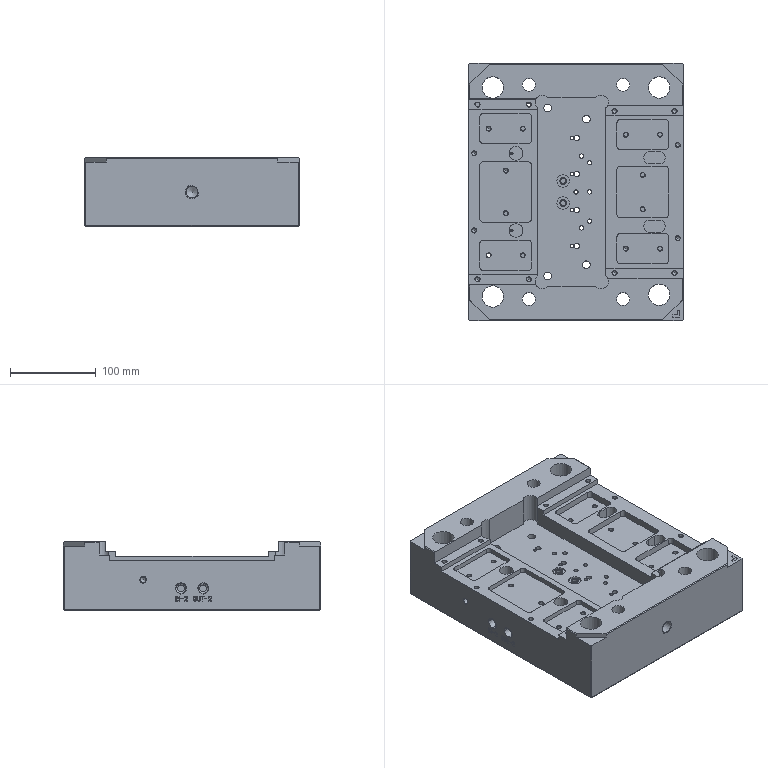NC program | PowerMill | posted with a generic post | part box 250 x 300 x 80 mm
Whole program:
%
O0001
N104 ( POWERMILL CB  : 2026004.0)
N105 ( POST VER      : 2026.0.0.5161)
N106 ( OPTION FILE   : FANUC)
N107 ( OUTPUT WORKPLANE : 2)
N108 (  )
N109 ( TOOL LIST )
N110 (-----------------------------------------)
N111 ( NO. | ID          | DIA.| TIP RAD|LENGTH)
N112 (-----------------------------------------)
N113 (    1|￠4中心钻_1_1| 4.0 |  0.0   |85.28 )
N114 (-----------------------------------------)
N115 (  )
N116 ( NUMBER OF TOOLPATHS: 1.0 )
N117 ( ESTIMATED PROGRAM DURATION: 0 HOURS 0 MIN 9 SEC)
N118 (  )
N119 G00 G21 G80 G40 G17
N120 G90
N121 G54
N122 G53 Z0.0
N123 (---------------)
N124 ( START TOOLPATH : 39开粗-￠4中心钻-打中心点 )
N125 (---------------)
N126 ( TOOL NO.    :1 )
N127 ( TOOL TYPE   : DRILL)
N128 ( TOOL ID     : ￠4中心钻_1_1)
N129 ( TOOL DIA    : 4.0 LENGTH 85.28)
N130 T1
N131 M6
N132 S3000 M03
N133 G00 G90 X-45.0 Y75.0
N134 G43 Z20.0 H1
N135
N136 G05 P10000 R8
N137 Z-34.7
N138 G01 Z-38.7 F60.0
N139 G00 Z20.0
N140 X45.0
N141 Z-34.7
N142 G01 Z-38.7
N143 G00 Z20.0
N144 G05 P0
N145 (---------------)
N146 ( END TOOLPATH : 39开粗-￠4中心钻-打中心点 )
N147 (---------------)
N148
N149 M05
N150 G53 Z0.0
N151 M30
%